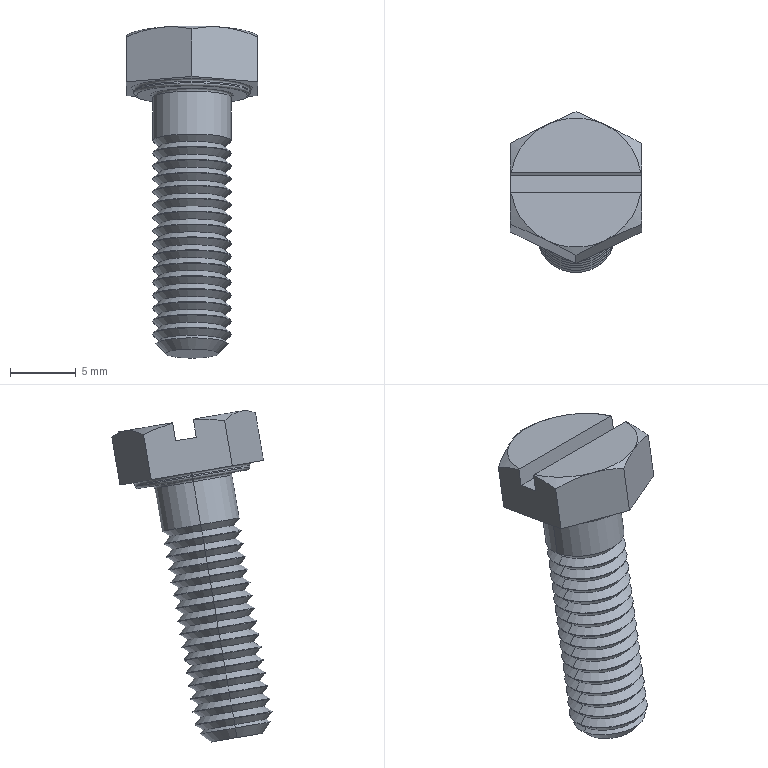Part | SolidWorks | features BaseBody 1 | 1 solid | 130 faces | box 10 x 12.249 x 25.328 mm | volume 840.877 mm3 | cone 72 | cylinder 34 | plane 18 | torus 6 | commonest cylinder face diameters 6 x32 8.88 x2